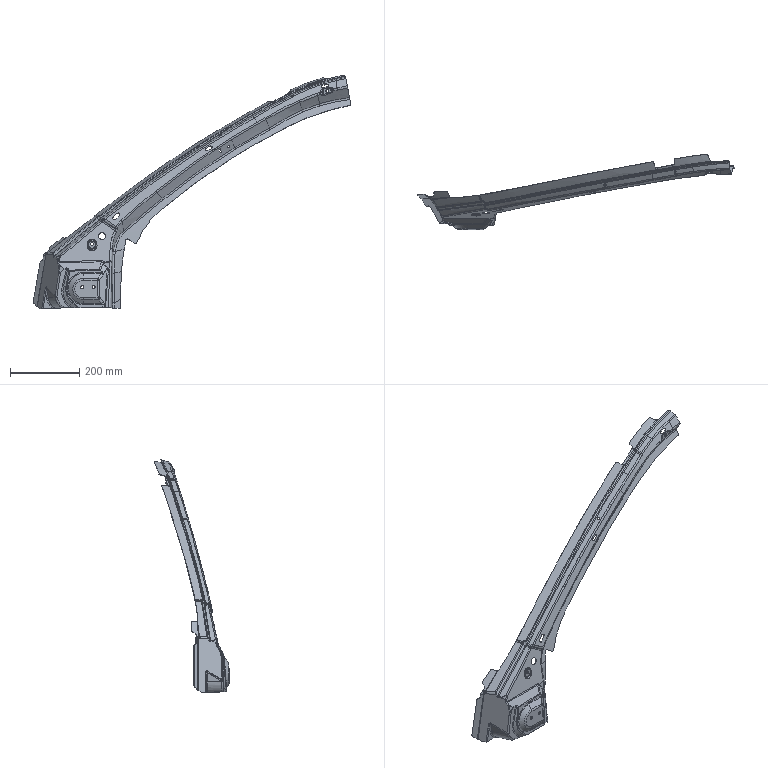Part | STEP file | FNA5401211 | 1 solid | 670 faces | box 914.927 x 216.551 x 677.274 mm | volume 215697 mm3 | spline 542 | cylinder 82 | plane 27 | sphere 14 | other 5 | commonest cylinder face diameters 12 x16 9.6 x12 16 x7 10 x6 13.6 x5 20 x5